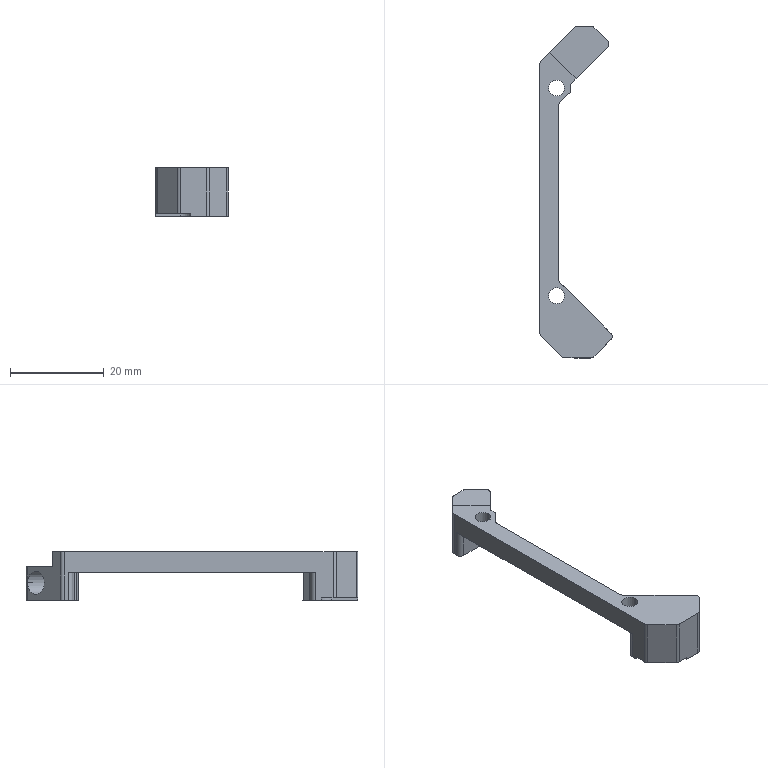Part | 1 solid | 62 faces | box 15.463 x 71 x 10.4 mm | volume 2578 mm3 | cylinder 31 | plane 27 | cone 4 | commonest cylinder face diameters 2 x20 3.4 x4 5.05 x2 5.2 x2 6.7 x2 4.4 x1